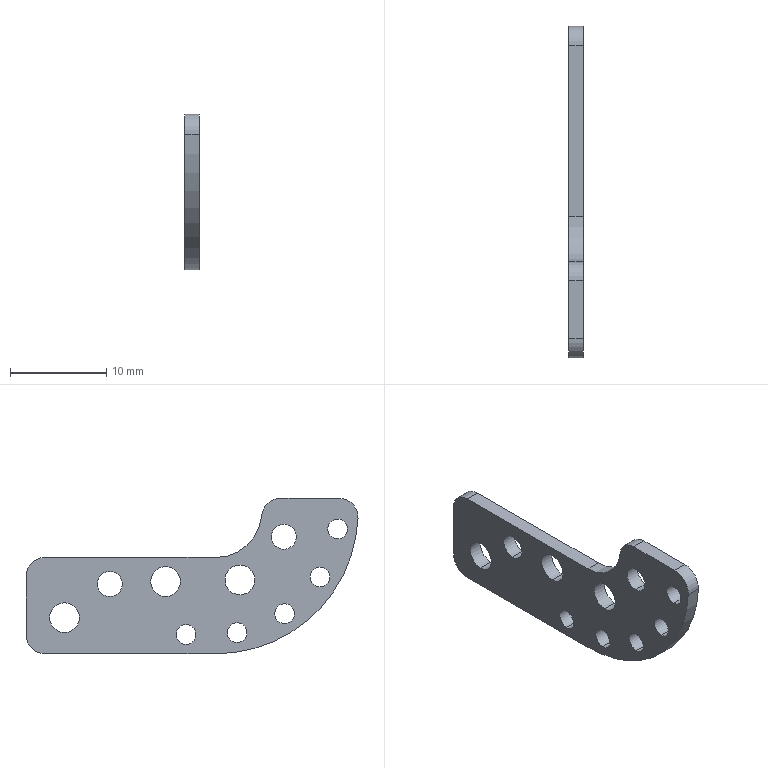Part | SolidWorks | features Extrusion 1, Fillet 1 | 1 solid | 32 faces | box 1.5 x 34.486 x 16.15 mm | volume 467.212 mm3 | cylinder 26 | plane 6 | commonest cylinder face diameters 2.05 x10 3.1 x6 2.6 x4 4 x4 9.5 x1 29.5 x1
STEP:
#1=CARTESIAN_POINT('',(1.5,5.25,15.2));
#2=VERTEX_POINT('',#1);
#3=CARTESIAN_POINT('',(1.5,5.25,18.3));
#4=VERTEX_POINT('',#3);
#5=CARTESIAN_POINT('',(1.5,5.25,16.75));
#6=DIRECTION('',(-1.,0.,0.));
#7=DIRECTION('',(0.,0.,-1.));
#8=AXIS2_PLACEMENT_3D('',#5,#6,#7);
#9=CIRCLE('',#8,1.55);
#10=EDGE_CURVE('',#2,#4,#9,.T.);
#11=ORIENTED_EDGE('',*,*,#10,.F.);
#12=CARTESIAN_POINT('',(0.,5.25,15.2));
#13=VERTEX_POINT('',#12);
#14=CARTESIAN_POINT('',(1.5,5.25,15.2));
#15=DIRECTION('',(-1.,0.,0.));
#16=VECTOR('',#15,1000.);
#17=LINE('',#14,#16);
#18=EDGE_CURVE('',#2,#13,#17,.T.);
#19=ORIENTED_EDGE('',*,*,#18,.T.);
#20=CARTESIAN_POINT('',(0.,5.25,18.3));
#21=VERTEX_POINT('',#20);
#22=CARTESIAN_POINT('',(0.,5.25,16.75));
#23=DIRECTION('',(-1.,0.,0.));
#24=DIRECTION('',(0.,0.,-1.));
#25=AXIS2_PLACEMENT_3D('',#22,#23,#24);
#26=CIRCLE('',#25,1.55);
#27=EDGE_CURVE('',#13,#21,#26,.T.);
#28=ORIENTED_EDGE('',*,*,#27,.T.);
#29=CARTESIAN_POINT('',(1.5,5.25,18.3));
#30=DIRECTION('',(-1.,0.,0.));
#31=VECTOR('',#30,1000.);
#32=LINE('',#29,#31);
#33=EDGE_CURVE('',#4,#21,#32,.T.);
#34=ORIENTED_EDGE('',*,*,#33,.F.);
#35=EDGE_LOOP('',(#11,#19,#28,#34));
#36=FACE_OUTER_BOUND('',#35,.T.);
#37=CARTESIAN_POINT('',(1.5,5.25,16.75));
#38=DIRECTION('',(-1.,0.,0.));
#39=DIRECTION('',(0.,0.,1.));
#40=AXIS2_PLACEMENT_3D('',#37,#38,#39);
#41=CYLINDRICAL_SURFACE('',#40,1.55);
#42=ADVANCED_FACE('',(#36),#41,.F.);
#43=CARTESIAN_POINT('',(1.5,15.75,14.55));
#44=VERTEX_POINT('',#43);
#45=CARTESIAN_POINT('',(1.5,15.75,11.45));
#46=VERTEX_POINT('',#45);
#47=CARTESIAN_POINT('',(1.5,15.75,13.));
#48=DIRECTION('',(1.,0.,0.));
#49=DIRECTION('',(0.,0.,-1.));
#50=AXIS2_PLACEMENT_3D('',#47,#48,#49);
#51=CIRCLE('',#50,1.55);
#52=EDGE_CURVE('',#44,#46,#51,.T.);
#53=ORIENTED_EDGE('',*,*,#52,.T.);
#54=CARTESIAN_POINT('',(0.,15.75,11.45));
#55=VERTEX_POINT('',#54);
#56=CARTESIAN_POINT('',(1.5,15.75,11.45));
#57=DIRECTION('',(-1.,0.,0.));
#58=VECTOR('',#57,1000.);
#59=LINE('',#56,#58);
#60=EDGE_CURVE('',#46,#55,#59,.T.);
#61=ORIENTED_EDGE('',*,*,#60,.T.);
#62=CARTESIAN_POINT('',(0.,15.75,14.55));
#63=VERTEX_POINT('',#62);
#64=CARTESIAN_POINT('',(0.,15.75,13.));
#65=DIRECTION('',(1.,0.,0.));
#66=DIRECTION('',(0.,0.,-1.));
#67=AXIS2_PLACEMENT_3D('',#64,#65,#66);
#68=CIRCLE('',#67,1.55);
#69=EDGE_CURVE('',#63,#55,#68,.T.);
#70=ORIENTED_EDGE('',*,*,#69,.F.);
#71=CARTESIAN_POINT('',(1.5,15.75,14.55));
#72=DIRECTION('',(-1.,0.,0.));
#73=VECTOR('',#72,1000.);
#74=LINE('',#71,#73);
#75=EDGE_CURVE('',#44,#63,#74,.T.);
#76=ORIENTED_EDGE('',*,*,#75,.F.);
#77=EDGE_LOOP('',(#53,#61,#70,#76));
#78=FACE_OUTER_BOUND('',#77,.T.);
#79=CARTESIAN_POINT('',(1.5,15.75,13.));
#80=DIRECTION('',(-1.,0.,0.));
#81=DIRECTION('',(0.,0.,1.));
#82=AXIS2_PLACEMENT_3D('',#79,#80,#81);
#83=CYLINDRICAL_SURFACE('',#82,1.55);
#84=ADVANCED_FACE('',(#78),#83,.F.);
#85=CARTESIAN_POINT('',(1.5,3.116,12.275));
#86=VERTEX_POINT('',#85);
#87=CARTESIAN_POINT('',(1.5,3.116,10.225));
#88=VERTEX_POINT('',#87);
#89=CARTESIAN_POINT('',(1.5,3.116,11.25));
#90=DIRECTION('',(1.,0.,0.));
#91=DIRECTION('',(0.,0.,-1.));
#92=AXIS2_PLACEMENT_3D('',#89,#90,#91);
#93=CIRCLE('',#92,1.025);
#94=EDGE_CURVE('',#86,#88,#93,.T.);
#95=ORIENTED_EDGE('',*,*,#94,.T.);
#96=CARTESIAN_POINT('',(0.,3.116,10.225));
#97=VERTEX_POINT('',#96);
#98=CARTESIAN_POINT('',(1.5,3.116,10.225));
#99=DIRECTION('',(-1.,0.,0.));
#100=VECTOR('',#99,1000.);
#101=LINE('',#98,#100);
#102=EDGE_CURVE('',#88,#97,#101,.T.);
#103=ORIENTED_EDGE('',*,*,#102,.T.);
#104=CARTESIAN_POINT('',(0.,3.116,12.275));
#105=VERTEX_POINT('',#104);
#106=CARTESIAN_POINT('',(0.,3.116,11.25));
#107=DIRECTION('',(1.,0.,0.));
#108=DIRECTION('',(0.,0.,-1.));
#109=AXIS2_PLACEMENT_3D('',#106,#107,#108);
#110=CIRCLE('',#109,1.025);
#111=EDGE_CURVE('',#105,#97,#110,.T.);
#112=ORIENTED_EDGE('',*,*,#111,.F.);
#113=CARTESIAN_POINT('',(1.5,3.116,12.275));
#114=DIRECTION('',(-1.,0.,0.));
#115=VECTOR('',#114,1000.);
#116=LINE('',#113,#115);
#117=EDGE_CURVE('',#86,#105,#116,.T.);
#118=ORIENTED_EDGE('',*,*,#117,.F.);
#119=EDGE_LOOP('',(#95,#103,#112,#118));
#120=FACE_OUTER_BOUND('',#119,.T.);
#121=CARTESIAN_POINT('',(1.5,3.116,11.25));
#122=DIRECTION('',(-1.,0.,0.));
#123=DIRECTION('',(0.,0.,1.));
#124=AXIS2_PLACEMENT_3D('',#121,#122,#123);
#125=CYLINDRICAL_SURFACE('',#124,1.025);
#126=ADVANCED_FACE('',(#120),#125,.F.);
#127=CARTESIAN_POINT('',(1.5,-12.621,23.219));
#128=VERTEX_POINT('',#127);
#129=CARTESIAN_POINT('',(1.5,-12.621,21.169));
#130=VERTEX_POINT('',#129);
#131=CARTESIAN_POINT('',(1.5,-12.621,22.194));
#132=DIRECTION('',(1.,0.,0.));
#133=DIRECTION('',(0.,0.,-1.));
#134=AXIS2_PLACEMENT_3D('',#131,#132,#133);
#135=CIRCLE('',#134,1.025);
#136=EDGE_CURVE('',#128,#130,#135,.T.);
#137=ORIENTED_EDGE('',*,*,#136,.T.);
#138=CARTESIAN_POINT('',(0.,-12.621,21.169));
#139=VERTEX_POINT('',#138);
#140=CARTESIAN_POINT('',(1.5,-12.621,21.169));
#141=DIRECTION('',(-1.,0.,0.));
#142=VECTOR('',#141,1000.);
#143=LINE('',#140,#142);
#144=EDGE_CURVE('',#130,#139,#143,.T.);
#145=ORIENTED_EDGE('',*,*,#144,.T.);
#146=CARTESIAN_POINT('',(0.,-12.621,23.219));
#147=VERTEX_POINT('',#146);
#148=CARTESIAN_POINT('',(0.,-12.621,22.194));
#149=DIRECTION('',(1.,0.,0.));
#150=DIRECTION('',(0.,0.,-1.));
#151=AXIS2_PLACEMENT_3D('',#148,#149,#150);
#152=CIRCLE('',#151,1.025);
#153=EDGE_CURVE('',#147,#139,#152,.T.);
#154=ORIENTED_EDGE('',*,*,#153,.F.);
#155=CARTESIAN_POINT('',(1.5,-12.621,23.219));
#156=DIRECTION('',(-1.,0.,0.));
#157=VECTOR('',#156,1000.);
#158=LINE('',#155,#157);
#159=EDGE_CURVE('',#128,#147,#158,.T.);
#160=ORIENTED_EDGE('',*,*,#159,.F.);
#161=EDGE_LOOP('',(#137,#145,#154,#160));
#162=FACE_OUTER_BOUND('',#161,.T.);
#163=CARTESIAN_POINT('',(1.5,-12.621,22.194));
#164=DIRECTION('',(-1.,0.,0.));
#165=DIRECTION('',(0.,0.,1.));
#166=AXIS2_PLACEMENT_3D('',#163,#164,#165);
#167=CYLINDRICAL_SURFACE('',#166,1.025);
#168=ADVANCED_FACE('',(#162),#167,.F.);
#169=CARTESIAN_POINT('',(1.5,-10.795,18.241));
#170=VERTEX_POINT('',#169);
#171=CARTESIAN_POINT('',(1.5,-10.795,16.191));
#172=VERTEX_POINT('',#171);
#173=CARTESIAN_POINT('',(1.5,-10.795,17.216));
#174=DIRECTION('',(1.,0.,0.));
#175=DIRECTION('',(0.,0.,-1.));
#176=AXIS2_PLACEMENT_3D('',#173,#174,#175);
#177=CIRCLE('',#176,1.025);
#178=EDGE_CURVE('',#170,#172,#177,.T.);
#179=ORIENTED_EDGE('',*,*,#178,.T.);
#180=CARTESIAN_POINT('',(0.,-10.795,16.191));
#181=VERTEX_POINT('',#180);
#182=CARTESIAN_POINT('',(1.5,-10.795,16.191));
#183=DIRECTION('',(-1.,0.,0.));
#184=VECTOR('',#183,1000.);
#185=LINE('',#182,#184);
#186=EDGE_CURVE('',#172,#181,#185,.T.);
#187=ORIENTED_EDGE('',*,*,#186,.T.);
#188=CARTESIAN_POINT('',(0.,-10.795,18.241));
#189=VERTEX_POINT('',#188);
#190=CARTESIAN_POINT('',(0.,-10.795,17.216));
#191=DIRECTION('',(1.,0.,0.));
#192=DIRECTION('',(0.,0.,-1.));
#193=AXIS2_PLACEMENT_3D('',#190,#191,#192);
#194=CIRCLE('',#193,1.025);
#195=EDGE_CURVE('',#189,#181,#194,.T.);
#196=ORIENTED_EDGE('',*,*,#195,.F.);
#197=CARTESIAN_POINT('',(1.5,-10.795,18.241));
#198=DIRECTION('',(-1.,0.,0.));
#199=VECTOR('',#198,1000.);
#200=LINE('',#197,#199);
#201=EDGE_CURVE('',#170,#189,#200,.T.);
#202=ORIENTED_EDGE('',*,*,#201,.F.);
#203=EDGE_LOOP('',(#179,#187,#196,#202));
#204=FACE_OUTER_BOUND('',#203,.T.);
#205=CARTESIAN_POINT('',(1.5,-10.795,17.216));
#206=DIRECTION('',(-1.,0.,0.));
#207=DIRECTION('',(0.,0.,1.));
#208=AXIS2_PLACEMENT_3D('',#205,#206,#207);
#209=CYLINDRICAL_SURFACE('',#208,1.025);
#210=ADVANCED_FACE('',(#204),#209,.F.);
#211=CARTESIAN_POINT('',(1.5,-7.103,14.437));
#212=VERTEX_POINT('',#211);
#213=CARTESIAN_POINT('',(1.5,-7.103,12.387));
#214=VERTEX_POINT('',#213);
#215=CARTESIAN_POINT('',(1.5,-7.103,13.412));
#216=DIRECTION('',(1.,0.,0.));
#217=DIRECTION('',(0.,0.,-1.));
#218=AXIS2_PLACEMENT_3D('',#215,#216,#217);
#219=CIRCLE('',#218,1.025);
#220=EDGE_CURVE('',#212,#214,#219,.T.);
#221=ORIENTED_EDGE('',*,*,#220,.T.);
#222=CARTESIAN_POINT('',(0.,-7.103,12.387));
#223=VERTEX_POINT('',#222);
#224=CARTESIAN_POINT('',(1.5,-7.103,12.387));
#225=DIRECTION('',(-1.,0.,0.));
#226=VECTOR('',#225,1000.);
#227=LINE('',#224,#226);
#228=EDGE_CURVE('',#214,#223,#227,.T.);
#229=ORIENTED_EDGE('',*,*,#228,.T.);
#230=CARTESIAN_POINT('',(0.,-7.103,14.437));
#231=VERTEX_POINT('',#230);
#232=CARTESIAN_POINT('',(0.,-7.103,13.412));
#233=DIRECTION('',(1.,0.,0.));
#234=DIRECTION('',(0.,0.,-1.));
#235=AXIS2_PLACEMENT_3D('',#232,#233,#234);
#236=CIRCLE('',#235,1.025);
#237=EDGE_CURVE('',#231,#223,#236,.T.);
#238=ORIENTED_EDGE('',*,*,#237,.F.);
#239=CARTESIAN_POINT('',(1.5,-7.103,14.437));
#240=DIRECTION('',(-1.,0.,0.));
#241=VECTOR('',#240,1000.);
#242=LINE('',#239,#241);
#243=EDGE_CURVE('',#212,#231,#242,.T.);
#244=ORIENTED_EDGE('',*,*,#243,.F.);
#245=EDGE_LOOP('',(#221,#229,#238,#244));
#246=FACE_OUTER_BOUND('',#245,.T.);
#247=CARTESIAN_POINT('',(1.5,-7.103,13.412));
#248=DIRECTION('',(-1.,0.,0.));
#249=DIRECTION('',(0.,0.,1.));
#250=AXIS2_PLACEMENT_3D('',#247,#248,#249);
#251=CYLINDRICAL_SURFACE('',#250,1.025);
#252=ADVANCED_FACE('',(#246),#251,.F.);
#253=CARTESIAN_POINT('',(1.5,-2.182,12.463));
#254=VERTEX_POINT('',#253);
#255=CARTESIAN_POINT('',(1.5,-2.182,10.413));
#256=VERTEX_POINT('',#255);
#257=CARTESIAN_POINT('',(1.5,-2.182,11.438));
#258=DIRECTION('',(1.,0.,0.));
#259=DIRECTION('',(0.,0.,-1.));
#260=AXIS2_PLACEMENT_3D('',#257,#258,#259);
#261=CIRCLE('',#260,1.025);
#262=EDGE_CURVE('',#254,#256,#261,.T.);
#263=ORIENTED_EDGE('',*,*,#262,.T.);
#264=CARTESIAN_POINT('',(0.,-2.182,10.413));
#265=VERTEX_POINT('',#264);
#266=CARTESIAN_POINT('',(1.5,-2.182,10.413));
#267=DIRECTION('',(-1.,0.,0.));
#268=VECTOR('',#267,1000.);
#269=LINE('',#266,#268);
#270=EDGE_CURVE('',#256,#265,#269,.T.);
#271=ORIENTED_EDGE('',*,*,#270,.T.);
#272=CARTESIAN_POINT('',(0.,-2.182,12.463));
#273=VERTEX_POINT('',#272);
#274=CARTESIAN_POINT('',(0.,-2.182,11.438));
#275=DIRECTION('',(1.,0.,0.));
#276=DIRECTION('',(0.,0.,-1.));
#277=AXIS2_PLACEMENT_3D('',#274,#275,#276);
#278=CIRCLE('',#277,1.025);
#279=EDGE_CURVE('',#273,#265,#278,.T.);
#280=ORIENTED_EDGE('',*,*,#279,.F.);
#281=CARTESIAN_POINT('',(1.5,-2.182,12.463));
#282=DIRECTION('',(-1.,0.,0.));
#283=VECTOR('',#282,1000.);
#284=LINE('',#281,#283);
#285=EDGE_CURVE('',#254,#273,#284,.T.);
#286=ORIENTED_EDGE('',*,*,#285,.F.);
#287=EDGE_LOOP('',(#263,#271,#280,#286));
#288=FACE_OUTER_BOUND('',#287,.T.);
#289=CARTESIAN_POINT('',(1.5,-2.182,11.438));
#290=DIRECTION('',(-1.,0.,0.));
#291=DIRECTION('',(0.,0.,1.));
#292=AXIS2_PLACEMENT_3D('',#289,#290,#291);
#293=CYLINDRICAL_SURFACE('',#292,1.025);
#294=ADVANCED_FACE('',(#288),#293,.F.);
#295=CARTESIAN_POINT('',(1.5,11.05,17.8));
#296=VERTEX_POINT('',#295);
#297=CARTESIAN_POINT('',(1.5,11.05,15.2));
#298=VERTEX_POINT('',#297);
#299=CARTESIAN_POINT('',(1.5,11.05,16.5));
#300=DIRECTION('',(1.,0.,0.));
#301=DIRECTION('',(0.,0.,-1.));
#302=AXIS2_PLACEMENT_3D('',#299,#300,#301);
#303=CIRCLE('',#302,1.3);
#304=EDGE_CURVE('',#296,#298,#303,.T.);
#305=ORIENTED_EDGE('',*,*,#304,.T.);
#306=CARTESIAN_POINT('',(0.,11.05,15.2));
#307=VERTEX_POINT('',#306);
#308=CARTESIAN_POINT('',(1.5,11.05,15.2));
#309=DIRECTION('',(-1.,0.,0.));
#310=VECTOR('',#309,1000.);
#311=LINE('',#308,#310);
#312=EDGE_CURVE('',#298,#307,#311,.T.);
#313=ORIENTED_EDGE('',*,*,#312,.T.);
#314=CARTESIAN_POINT('',(0.,11.05,17.8));
#315=VERTEX_POINT('',#314);
#316=CARTESIAN_POINT('',(0.,11.05,16.5));
#317=DIRECTION('',(1.,0.,0.));
#318=DIRECTION('',(0.,0.,-1.));
#319=AXIS2_PLACEMENT_3D('',#316,#317,#318);
#320=CIRCLE('',#319,1.3);
#321=EDGE_CURVE('',#315,#307,#320,.T.);
#322=ORIENTED_EDGE('',*,*,#321,.F.);
#323=CARTESIAN_POINT('',(1.5,11.05,17.8));
#324=DIRECTION('',(-1.,0.,0.));
#325=VECTOR('',#324,1000.);
#326=LINE('',#323,#325);
#327=EDGE_CURVE('',#296,#315,#326,.T.);
#328=ORIENTED_EDGE('',*,*,#327,.F.);
#329=EDGE_LOOP('',(#305,#313,#322,#328));
#330=FACE_OUTER_BOUND('',#329,.T.);
#331=CARTESIAN_POINT('',(1.5,11.05,16.5));
#332=DIRECTION('',(-1.,0.,0.));
#333=DIRECTION('',(0.,0.,1.));
#334=AXIS2_PLACEMENT_3D('',#331,#332,#333);
#335=CYLINDRICAL_SURFACE('',#334,1.3);
#336=ADVANCED_FACE('',(#330),#335,.F.);
#337=CARTESIAN_POINT('',(1.5,-7.035,22.7));
#338=VERTEX_POINT('',#337);
#339=CARTESIAN_POINT('',(1.5,-7.035,20.1));
#340=VERTEX_POINT('',#339);
#341=CARTESIAN_POINT('',(1.5,-7.035,21.4));
#342=DIRECTION('',(1.,0.,0.));
#343=DIRECTION('',(0.,0.,-1.));
#344=AXIS2_PLACEMENT_3D('',#341,#342,#343);
#345=CIRCLE('',#344,1.3);
#346=EDGE_CURVE('',#338,#340,#345,.T.);
#347=ORIENTED_EDGE('',*,*,#346,.T.);
#348=CARTESIAN_POINT('',(0.,-7.035,20.1));
#349=VERTEX_POINT('',#348);
#350=CARTESIAN_POINT('',(1.5,-7.035,20.1));
#351=DIRECTION('',(-1.,0.,0.));
#352=VECTOR('',#351,1000.);
#353=LINE('',#350,#352);
#354=EDGE_CURVE('',#340,#349,#353,.T.);
#355=ORIENTED_EDGE('',*,*,#354,.T.);
#356=CARTESIAN_POINT('',(0.,-7.035,22.7));
#357=VERTEX_POINT('',#356);
#358=CARTESIAN_POINT('',(0.,-7.035,21.4));
#359=DIRECTION('',(1.,0.,0.));
#360=DIRECTION('',(0.,0.,-1.));
#361=AXIS2_PLACEMENT_3D('',#358,#359,#360);
#362=CIRCLE('',#361,1.3);
#363=EDGE_CURVE('',#357,#349,#362,.T.);
#364=ORIENTED_EDGE('',*,*,#363,.F.);
#365=CARTESIAN_POINT('',(1.5,-7.035,22.7));
#366=DIRECTION('',(-1.,0.,0.));
#367=VECTOR('',#366,1000.);
#368=LINE('',#365,#367);
#369=EDGE_CURVE('',#338,#357,#368,.T.);
#370=ORIENTED_EDGE('',*,*,#369,.F.);
#371=EDGE_LOOP('',(#347,#355,#364,#370));
#372=FACE_OUTER_BOUND('',#371,.T.);
#373=CARTESIAN_POINT('',(1.5,-7.035,21.4));
#374=DIRECTION('',(-1.,0.,0.));
#375=DIRECTION('',(0.,0.,1.));
#376=AXIS2_PLACEMENT_3D('',#373,#374,#375);
#377=CYLINDRICAL_SURFACE('',#376,1.3);
#378=ADVANCED_FACE('',(#372),#377,.F.);
#379=CARTESIAN_POINT('',(1.5,-2.467,18.467));
#380=VERTEX_POINT('',#379);
#381=CARTESIAN_POINT('',(1.5,-2.467,15.367));
#382=VERTEX_POINT('',#381);
#383=CARTESIAN_POINT('',(1.5,-2.467,16.917));
#384=DIRECTION('',(1.,0.,0.));
#385=DIRECTION('',(0.,0.,-1.));
#386=AXIS2_PLACEMENT_3D('',#383,#384,#385);
#387=CIRCLE('',#386,1.55);
#388=EDGE_CURVE('',#380,#382,#387,.T.);
#389=ORIENTED_EDGE('',*,*,#388,.T.);
#390=CARTESIAN_POINT('',(0.,-2.467,15.367));
#391=VERTEX_POINT('',#390);
#392=CARTESIAN_POINT('',(1.5,-2.467,15.367));
#393=DIRECTION('',(-1.,0.,0.));
#394=VECTOR('',#393,1000.);
#395=LINE('',#392,#394);
#396=EDGE_CURVE('',#382,#391,#395,.T.);
#397=ORIENTED_EDGE('',*,*,#396,.T.);
#398=CARTESIAN_POINT('',(0.,-2.467,18.467));
#399=VERTEX_POINT('',#398);
#400=CARTESIAN_POINT('',(0.,-2.467,16.917));
#401=DIRECTION('',(1.,0.,0.));
#402=DIRECTION('',(0.,0.,-1.));
#403=AXIS2_PLACEMENT_3D('',#400,#401,#402);
#404=CIRCLE('',#403,1.55);
#405=EDGE_CURVE('',#399,#391,#404,.T.);
#406=ORIENTED_EDGE('',*,*,#405,.F.);
#407=CARTESIAN_POINT('',(1.5,-2.467,18.467));
#408=DIRECTION('',(-1.,0.,0.));
#409=VECTOR('',#408,1000.);
#410=LINE('',#407,#409);
#411=EDGE_CURVE('',#380,#399,#410,.T.);
#412=ORIENTED_EDGE('',*,*,#411,.F.);
#413=EDGE_LOOP('',(#389,#397,#406,#412));
#414=FACE_OUTER_BOUND('',#413,.T.);
#415=CARTESIAN_POINT('',(1.5,-2.467,16.917));
#416=DIRECTION('',(-1.,0.,0.));
#417=DIRECTION('',(0.,0.,1.));
#418=AXIS2_PLACEMENT_3D('',#415,#416,#417);
#419=CYLINDRICAL_SURFACE('',#418,1.55);
#420=ADVANCED_FACE('',(#414),#419,.F.);
#421=CARTESIAN_POINT('',(0.,0.,9.25));
#422=VERTEX_POINT('',#421);
#423=CARTESIAN_POINT('',(0.,17.75,9.25));
#424=VERTEX_POINT('',#423);
#425=CARTESIAN_POINT('',(0.,0.,9.25));
#426=DIRECTION('',(0.,1.,0.));
#427=VECTOR('',#426,1000.);
#428=LINE('',#425,#427);
#429=EDGE_CURVE('',#422,#424,#428,.T.);
#430=ORIENTED_EDGE('',*,*,#429,.T.);
#431=CARTESIAN_POINT('',(1.5,17.75,9.25));
#432=VERTEX_POINT('',#431);
#433=CARTESIAN_POINT('',(1.5,17.75,9.25));
#434=DIRECTION('',(1.,0.,0.));
#435=VECTOR('',#434,1000.);
#436=LINE('',#433,#435);
#437=EDGE_CURVE('',#424,#432,#436,.T.);
#438=ORIENTED_EDGE('',*,*,#437,.T.);
#439=CARTESIAN_POINT('',(1.5,0.,9.25));
#440=VERTEX_POINT('',#439);
#441=CARTESIAN_POINT('',(1.5,0.,9.25));
#442=DIRECTION('',(0.,1.,0.));
#443=VECTOR('',#442,1000.);
#444=LINE('',#441,#443);
#445=EDGE_CURVE('',#440,#432,#444,.T.);
#446=ORIENTED_EDGE('',*,*,#445,.F.);
#447=CARTESIAN_POINT('',(1.5,0.,9.25));
#448=DIRECTION('',(-1.,0.,0.));
#449=VECTOR('',#448,1000.);
#450=LINE('',#447,#449);
#451=EDGE_CURVE('',#440,#422,#450,.T.);
#452=ORIENTED_EDGE('',*,*,#451,.T.);
#453=EDGE_LOOP('',(#430,#438,#446,#452));
#454=FACE_OUTER_BOUND('',#453,.T.);
#455=CARTESIAN_POINT('',(1.5,0.,9.25));
#456=DIRECTION('',(0.,0.,1.));
#457=DIRECTION('',(1.,0.,0.));
#458=AXIS2_PLACEMENT_3D('',#455,#456,#457);
#459=PLANE('',#458);
#460=ADVANCED_FACE('',(#454),#459,.F.);
#461=CARTESIAN_POINT('',(0.,19.75,17.25));
#462=VERTEX_POINT('',#461);
#463=CARTESIAN_POINT('',(0.,19.75,11.25));
#464=VERTEX_POINT('',#463);
#465=CARTESIAN_POINT('',(0.,19.75,0.));
#466=DIRECTION('',(0.,0.,-1.));
#467=VECTOR('',#466,1000.);
#468=LINE('',#465,#467);
#469=EDGE_CURVE('',#462,#464,#468,.T.);
#470=ORIENTED_EDGE('',*,*,#469,.F.);
#471=CARTESIAN_POINT('',(1.5,19.75,17.25));
#472=VERTEX_POINT('',#471);
#473=CARTESIAN_POINT('',(1.5,19.75,17.25));
#474=DIRECTION('',(1.,0.,0.));
#475=VECTOR('',#474,1000.);
#476=LINE('',#473,#475);
#477=EDGE_CURVE('',#462,#472,#476,.T.);
#478=ORIENTED_EDGE('',*,*,#477,.T.);
#479=CARTESIAN_POINT('',(1.5,19.75,11.25));
#480=VERTEX_POINT('',#479);
#481=CARTESIAN_POINT('',(1.5,19.75,0.));
#482=DIRECTION('',(0.,0.,-1.));
#483=VECTOR('',#482,1000.);
#484=LINE('',#481,#483);
#485=EDGE_CURVE('',#472,#480,#484,.T.);
#486=ORIENTED_EDGE('',*,*,#485,.T.);
#487=CARTESIAN_POINT('',(0.,19.75,11.25));
#488=DIRECTION('',(-1.,0.,0.));
#489=VECTOR('',#488,1000.);
#490=LINE('',#487,#489);
#491=EDGE_CURVE('',#480,#464,#490,.T.);
#492=ORIENTED_EDGE('',*,*,#491,.T.);
#493=EDGE_LOOP('',(#470,#478,#486,#492));
#494=FACE_OUTER_BOUND('',#493,.T.);
#495=CARTESIAN_POINT('',(1.5,19.75,0.));
#496=DIRECTION('',(0.,1.,0.));
#497=DIRECTION('',(0.,0.,1.));
#498=AXIS2_PLACEMENT_3D('',#495,#496,#497);
#499=PLANE('',#498);
#500=ADVANCED_FACE('',(#494),#499,.T.);
#501=CARTESIAN_POINT('',(1.5,0.,19.25));
#502=VERTEX_POINT('',#501);
#503=CARTESIAN_POINT('',(1.5,17.75,19.25));
#504=VERTEX_POINT('',#503);
#505=CARTESIAN_POINT('',(1.5,0.,19.25));
#506=DIRECTION('',(0.,1.,0.));
#507=VECTOR('',#506,1000.);
#508=LINE('',#505,#507);
#509=EDGE_CURVE('',#502,#504,#508,.T.);
#510=ORIENTED_EDGE('',*,*,#509,.T.);
#511=CARTESIAN_POINT('',(0.,17.75,19.25));
#512=VERTEX_POINT('',#511);
#513=CARTESIAN_POINT('',(1.5,17.75,19.25));
#514=DIRECTION('',(-1.,0.,0.));
#515=VECTOR('',#514,1000.);
#516=LINE('',#513,#515);
#517=EDGE_CURVE('',#504,#512,#516,.T.);
#518=ORIENTED_EDGE('',*,*,#517,.T.);
#519=CARTESIAN_POINT('',(0.,0.,19.25));
#520=VERTEX_POINT('',#519);
#521=CARTESIAN_POINT('',(0.,0.,19.25));
#522=DIRECTION('',(0.,1.,0.));
#523=VECTOR('',#522,1000.);
#524=LINE('',#521,#523);
#525=EDGE_CURVE('',#520,#512,#524,.T.);
#526=ORIENTED_EDGE('',*,*,#525,.F.);
#527=CARTESIAN_POINT('',(1.5,0.,19.25));
#528=DIRECTION('',(-1.,0.,0.));
#529=VECTOR('',#528,1000.);
#530=LINE('',#527,#529);
#531=EDGE_CURVE('',#502,#520,#530,.T.);
#532=ORIENTED_EDGE('',*,*,#531,.F.);
#533=EDGE_LOOP('',(#510,#518,#526,#532));
#534=FACE_OUTER_BOUND('',#533,.T.);
#535=CARTESIAN_POINT('',(1.5,0.,19.25));
#536=DIRECTION('',(0.,0.,1.));
#537=DIRECTION('',(0.,-1.,0.));
#538=AXIS2_PLACEMENT_3D('',#535,#536,#537);
#539=PLANE('',#538);
#540=ADVANCED_FACE('',(#534),#539,.T.);
#541=CARTESIAN_POINT('',(0.,-4.731,23.578));
#542=VERTEX_POINT('',#541);
#543=CARTESIAN_POINT('',(0.,0.,24.));
#544=DIRECTION('',(1.,0.,0.));
#545=DIRECTION('',(0.,0.,-1.));
#546=AXIS2_PLACEMENT_3D('',#543,#544,#545);
#547=CIRCLE('',#546,4.75);
#548=EDGE_CURVE('',#542,#520,#547,.T.);
#549=ORIENTED_EDGE('',*,*,#548,.F.);
#550=CARTESIAN_POINT('',(1.5,-4.731,23.578));
#551=VERTEX_POINT('',#550);
#552=CARTESIAN_POINT('',(1.5,-4.731,23.578));
#553=DIRECTION('',(1.,0.,0.));
#554=VECTOR('',#553,1000.);
#555=LINE('',#552,#554);
#556=EDGE_CURVE('',#542,#551,#555,.T.);
#557=ORIENTED_EDGE('',*,*,#556,.T.);
#558=CARTESIAN_POINT('',(1.5,0.,24.));
#559=DIRECTION('',(1.,0.,0.));
#560=DIRECTION('',(0.,0.,-1.));
#561=AXIS2_PLACEMENT_3D('',#558,#559,#560);
#562=CIRCLE('',#561,4.75);
#563=EDGE_CURVE('',#551,#502,#562,.T.);
#564=ORIENTED_EDGE('',*,*,#563,.T.);
#565=ORIENTED_EDGE('',*,*,#531,.T.);
#566=EDGE_LOOP('',(#549,#557,#564,#565));
#567=FACE_OUTER_BOUND('',#566,.T.);
#568=CARTESIAN_POINT('',(1.5,0.,24.));
#569=DIRECTION('',(-1.,0.,0.));
#570=DIRECTION('',(0.,0.,1.));
#571=AXIS2_PLACEMENT_3D('',#568,#569,#570);
#572=CYLINDRICAL_SURFACE('',#571,4.75);
#573=ADVANCED_FACE('',(#567),#572,.F.);
#574=CARTESIAN_POINT('',(1.5,-6.723,25.4));
#575=VERTEX_POINT('',#574);
#576=CARTESIAN_POINT('',(1.5,-12.736,25.4));
#577=VERTEX_POINT('',#576);
#578=CARTESIAN_POINT('',(1.5,0.,25.4));
#579=DIRECTION('',(0.,-1.,0.));
#580=VECTOR('',#579,1000.);
#581=LINE('',#578,#580);
#582=EDGE_CURVE('',#575,#577,#581,.T.);
#583=ORIENTED_EDGE('',*,*,#582,.F.);
#584=CARTESIAN_POINT('',(0.,-6.723,25.4));
#585=VERTEX_POINT('',#584);
#586=CARTESIAN_POINT('',(0.,-6.723,25.4));
#587=DIRECTION('',(-1.,0.,0.));
#588=VECTOR('',#587,1000.);
#589=LINE('',#586,#588);
#590=EDGE_CURVE('',#575,#585,#589,.T.);
#591=ORIENTED_EDGE('',*,*,#590,.T.);
#592=CARTESIAN_POINT('',(0.,-12.736,25.4));
#593=VERTEX_POINT('',#592);
#594=CARTESIAN_POINT('',(0.,0.,25.4));
#595=DIRECTION('',(0.,-1.,0.));
#596=VECTOR('',#595,1000.);
#597=LINE('',#594,#596);
#598=EDGE_CURVE('',#585,#593,#597,.T.);
#599=ORIENTED_EDGE('',*,*,#598,.T.);
#600=CARTESIAN_POINT('',(1.5,-12.736,25.4));
#601=DIRECTION('',(1.,0.,0.));
#602=VECTOR('',#601,1000.);
#603=LINE('',#600,#602);
#604=EDGE_CURVE('',#593,#577,#603,.T.);
#605=ORIENTED_EDGE('',*,*,#604,.T.);
#606=EDGE_LOOP('',(#583,#591,#599,#605));
#607=FACE_OUTER_BOUND('',#606,.T.);
#608=CARTESIAN_POINT('',(1.5,0.,25.4));
#609=DIRECTION('',(0.,0.,-1.));
#610=DIRECTION('',(0.,1.,0.));
#611=AXIS2_PLACEMENT_3D('',#608,#609,#610);
#612=PLANE('',#611);
#613=ADVANCED_FACE('',(#607),#612,.F.);
#614=ORIENTED_EDGE('',*,*,#396,.F.);
#615=CARTESIAN_POINT('',(1.5,-2.467,16.917));
#616=DIRECTION('',(1.,0.,0.));
#617=DIRECTION('',(0.,0.,-1.));
#618=AXIS2_PLACEMENT_3D('',#615,#616,#617);
#619=CIRCLE('',#618,1.55);
#620=EDGE_CURVE('',#382,#380,#619,.T.);
#621=ORIENTED_EDGE('',*,*,#620,.T.);
#622=ORIENTED_EDGE('',*,*,#411,.T.);
#623=CARTESIAN_POINT('',(0.,-2.467,16.917));
#624=DIRECTION('',(1.,0.,0.));
#625=DIRECTION('',(0.,0.,-1.));
#626=AXIS2_PLACEMENT_3D('',#623,#624,#625);
#627=CIRCLE('',#626,1.55);
#628=EDGE_CURVE('',#391,#399,#627,.T.);
#629=ORIENTED_EDGE('',*,*,#628,.F.);
#630=EDGE_LOOP('',(#614,#621,#622,#629));
#631=FACE_OUTER_BOUND('',#630,.T.);
#632=CARTESIAN_POINT('',(1.5,-2.467,16.917));
#633=DIRECTION('',(-1.,0.,0.));
#634=DIRECTION('',(0.,0.,1.));
#635=AXIS2_PLACEMENT_3D('',#632,#633,#634);
#636=CYLINDRICAL_SURFACE('',#635,1.55);
#637=ADVANCED_FACE('',(#631),#636,.F.);
#638=ORIENTED_EDGE('',*,*,#354,.F.);
#639=CARTESIAN_POINT('',(1.5,-7.035,21.4));
#640=DIRECTION('',(1.,0.,0.));
#641=DIRECTION('',(0.,0.,-1.));
#642=AXIS2_PLACEMENT_3D('',#639,#640,#641);
#643=CIRCLE('',#642,1.3);
#644=EDGE_CURVE('',#340,#338,#643,.T.);
#645=ORIENTED_EDGE('',*,*,#644,.T.);
#646=ORIENTED_EDGE('',*,*,#369,.T.);
#647=CARTESIAN_POINT('',(0.,-7.035,21.4));
#648=DIRECTION('',(1.,0.,0.));
#649=DIRECTION('',(0.,0.,-1.));
#650=AXIS2_PLACEMENT_3D('',#647,#648,#649);
#651=CIRCLE('',#650,1.3);
#652=EDGE_CURVE('',#349,#357,#651,.T.);
#653=ORIENTED_EDGE('',*,*,#652,.F.);
#654=EDGE_LOOP('',(#638,#645,#646,#653));
#655=FACE_OUTER_BOUND('',#654,.T.);
#656=CARTESIAN_POINT('',(1.5,-7.035,21.4));
#657=DIRECTION('',(-1.,0.,0.));
#658=DIRECTION('',(0.,0.,1.));
#659=AXIS2_PLACEMENT_3D('',#656,#657,#658);
#660=CYLINDRICAL_SURFACE('',#659,1.3);
#661=ADVANCED_FACE('',(#655),#660,.F.);
#662=ORIENTED_EDGE('',*,*,#312,.F.);
#663=CARTESIAN_POINT('',(1.5,11.05,16.5));
#664=DIRECTION('',(1.,0.,0.));
#665=DIRECTION('',(0.,0.,-1.));
#666=AXIS2_PLACEMENT_3D('',#663,#664,#665);
#667=CIRCLE('',#666,1.3);
#668=EDGE_CURVE('',#298,#296,#667,.T.);
#669=ORIENTED_EDGE('',*,*,#668,.T.);
#670=ORIENTED_EDGE('',*,*,#327,.T.);
#671=CARTESIAN_POINT('',(0.,11.05,16.5));
#672=DIRECTION('',(1.,0.,0.));
#673=DIRECTION('',(0.,0.,-1.));
#674=AXIS2_PLACEMENT_3D('',#671,#672,#673);
#675=CIRCLE('',#674,1.3);
#676=EDGE_CURVE('',#307,#315,#675,.T.);
#677=ORIENTED_EDGE('',*,*,#676,.F.);
#678=EDGE_LOOP('',(#662,#669,#670,#677));
#679=FACE_OUTER_BOUND('',#678,.T.);
#680=CARTESIAN_POINT('',(1.5,11.05,16.5));
#681=DIRECTION('',(-1.,0.,0.));
#682=DIRECTION('',(0.,0.,1.));
#683=AXIS2_PLACEMENT_3D('',#680,#681,#682);
#684=CYLINDRICAL_SURFACE('',#683,1.3);
#685=ADVANCED_FACE('',(#679),#684,.F.);
#686=ORIENTED_EDGE('',*,*,#270,.F.);
#687=CARTESIAN_POINT('',(1.5,-2.182,11.438));
#688=DIRECTION('',(1.,0.,0.));
#689=DIRECTION('',(0.,0.,-1.));
#690=AXIS2_PLACEMENT_3D('',#687,#688,#689);
#691=CIRCLE('',#690,1.025);
#692=EDGE_CURVE('',#256,#254,#691,.T.);
#693=ORIENTED_EDGE('',*,*,#692,.T.);
#694=ORIENTED_EDGE('',*,*,#285,.T.);
#695=CARTESIAN_POINT('',(0.,-2.182,11.438));
#696=DIRECTION('',(1.,0.,0.));
#697=DIRECTION('',(0.,0.,-1.));
#698=AXIS2_PLACEMENT_3D('',#695,#696,#697);
#699=CIRCLE('',#698,1.025);
#700=EDGE_CURVE('',#265,#273,#699,.T.);
#701=ORIENTED_EDGE('',*,*,#700,.F.);
#702=EDGE_LOOP('',(#686,#693,#694,#701));
#703=FACE_OUTER_BOUND('',#702,.T.);
#704=CARTESIAN_POINT('',(1.5,-2.182,11.438));
#705=DIRECTION('',(-1.,0.,0.));
#706=DIRECTION('',(0.,0.,1.));
#707=AXIS2_PLACEMENT_3D('',#704,#705,#706);
#708=CYLINDRICAL_SURFACE('',#707,1.025);
#709=ADVANCED_FACE('',(#703),#708,.F.);
#710=ORIENTED_EDGE('',*,*,#228,.F.);
#711=CARTESIAN_POINT('',(1.5,-7.103,13.412));
#712=DIRECTION('',(1.,0.,0.));
#713=DIRECTION('',(0.,0.,-1.));
#714=AXIS2_PLACEMENT_3D('',#711,#712,#713);
#715=CIRCLE('',#714,1.025);
#716=EDGE_CURVE('',#214,#212,#715,.T.);
#717=ORIENTED_EDGE('',*,*,#716,.T.);
#718=ORIENTED_EDGE('',*,*,#243,.T.);
#719=CARTESIAN_POINT('',(0.,-7.103,13.412));
#720=DIRECTION('',(1.,0.,0.));
#721=DIRECTION('',(0.,0.,-1.));
#722=AXIS2_PLACEMENT_3D('',#719,#720,#721);
#723=CIRCLE('',#722,1.025);
#724=EDGE_CURVE('',#223,#231,#723,.T.);
#725=ORIENTED_EDGE('',*,*,#724,.F.);
#726=EDGE_LOOP('',(#710,#717,#718,#725));
#727=FACE_OUTER_BOUND('',#726,.T.);
#728=CARTESIAN_POINT('',(1.5,-7.103,13.412));
#729=DIRECTION('',(-1.,0.,0.));
#730=DIRECTION('',(0.,0.,1.));
#731=AXIS2_PLACEMENT_3D('',#728,#729,#730);
#732=CYLINDRICAL_SURFACE('',#731,1.025);
#733=ADVANCED_FACE('',(#727),#732,.F.);
#734=ORIENTED_EDGE('',*,*,#186,.F.);
#735=CARTESIAN_POINT('',(1.5,-10.795,17.216));
#736=DIRECTION('',(1.,0.,0.));
#737=DIRECTION('',(0.,0.,-1.));
#738=AXIS2_PLACEMENT_3D('',#735,#736,#737);
#739=CIRCLE('',#738,1.025);
#740=EDGE_CURVE('',#172,#170,#739,.T.);
#741=ORIENTED_EDGE('',*,*,#740,.T.);
#742=ORIENTED_EDGE('',*,*,#201,.T.);
#743=CARTESIAN_POINT('',(0.,-10.795,17.216));
#744=DIRECTION('',(1.,0.,0.));
#745=DIRECTION('',(0.,0.,-1.));
#746=AXIS2_PLACEMENT_3D('',#743,#744,#745);
#747=CIRCLE('',#746,1.025);
#748=EDGE_CURVE('',#181,#189,#747,.T.);
#749=ORIENTED_EDGE('',*,*,#748,.F.);
#750=EDGE_LOOP('',(#734,#741,#742,#749));
#751=FACE_OUTER_BOUND('',#750,.T.);
#752=CARTESIAN_POINT('',(1.5,-10.795,17.216));
#753=DIRECTION('',(-1.,0.,0.));
#754=DIRECTION('',(0.,0.,1.));
#755=AXIS2_PLACEMENT_3D('',#752,#753,#754);
#756=CYLINDRICAL_SURFACE('',#755,1.025);
#757=ADVANCED_FACE('',(#751),#756,.F.);
#758=ORIENTED_EDGE('',*,*,#144,.F.);
#759=CARTESIAN_POINT('',(1.5,-12.621,22.194));
#760=DIRECTION('',(1.,0.,0.));
#761=DIRECTION('',(0.,0.,-1.));
#762=AXIS2_PLACEMENT_3D('',#759,#760,#761);
#763=CIRCLE('',#762,1.025);
#764=EDGE_CURVE('',#130,#128,#763,.T.);
#765=ORIENTED_EDGE('',*,*,#764,.T.);
#766=ORIENTED_EDGE('',*,*,#159,.T.);
#767=CARTESIAN_POINT('',(0.,-12.621,22.194));
#768=DIRECTION('',(1.,0.,0.));
#769=DIRECTION('',(0.,0.,-1.));
#770=AXIS2_PLACEMENT_3D('',#767,#768,#769);
#771=CIRCLE('',#770,1.025);
#772=EDGE_CURVE('',#139,#147,#771,.T.);
#773=ORIENTED_EDGE('',*,*,#772,.F.);
#774=EDGE_LOOP('',(#758,#765,#766,#773));
#775=FACE_OUTER_BOUND('',#774,.T.);
#776=CARTESIAN_POINT('',(1.5,-12.621,22.194));
#777=DIRECTION('',(-1.,0.,0.));
#778=DIRECTION('',(0.,0.,1.));
#779=AXIS2_PLACEMENT_3D('',#776,#777,#778);
#780=CYLINDRICAL_SURFACE('',#779,1.025);
#781=ADVANCED_FACE('',(#775),#780,.F.);
#782=ORIENTED_EDGE('',*,*,#102,.F.);
#783=CARTESIAN_POINT('',(1.5,3.116,11.25));
#784=DIRECTION('',(1.,0.,0.));
#785=DIRECTION('',(0.,0.,-1.));
#786=AXIS2_PLACEMENT_3D('',#783,#784,#785);
#787=CIRCLE('',#786,1.025);
#788=EDGE_CURVE('',#88,#86,#787,.T.);
#789=ORIENTED_EDGE('',*,*,#788,.T.);
#790=ORIENTED_EDGE('',*,*,#117,.T.);
#791=CARTESIAN_POINT('',(0.,3.116,11.25));
#792=DIRECTION('',(1.,0.,0.));
#793=DIRECTION('',(0.,0.,-1.));
#794=AXIS2_PLACEMENT_3D('',#791,#792,#793);
#795=CIRCLE('',#794,1.025);
#796=EDGE_CURVE('',#97,#105,#795,.T.);
#797=ORIENTED_EDGE('',*,*,#796,.F.);
#798=EDGE_LOOP('',(#782,#789,#790,#797));
#799=FACE_OUTER_BOUND('',#798,.T.);
#800=CARTESIAN_POINT('',(1.5,3.116,11.25));
#801=DIRECTION('',(-1.,0.,0.));
#802=DIRECTION('',(0.,0.,1.));
#803=AXIS2_PLACEMENT_3D('',#800,#801,#802);
#804=CYLINDRICAL_SURFACE('',#803,1.025);
#805=ADVANCED_FACE('',(#799),#804,.F.);
#806=ORIENTED_EDGE('',*,*,#60,.F.);
#807=CARTESIAN_POINT('',(1.5,15.75,13.));
#808=DIRECTION('',(1.,0.,0.));
#809=DIRECTION('',(0.,0.,-1.));
#810=AXIS2_PLACEMENT_3D('',#807,#808,#809);
#811=CIRCLE('',#810,1.55);
#812=EDGE_CURVE('',#46,#44,#811,.T.);
#813=ORIENTED_EDGE('',*,*,#812,.T.);
#814=ORIENTED_EDGE('',*,*,#75,.T.);
#815=CARTESIAN_POINT('',(0.,15.75,13.));
#816=DIRECTION('',(1.,0.,0.));
#817=DIRECTION('',(0.,0.,-1.));
#818=AXIS2_PLACEMENT_3D('',#815,#816,#817);
#819=CIRCLE('',#818,1.55);
#820=EDGE_CURVE('',#55,#63,#819,.T.);
#821=ORIENTED_EDGE('',*,*,#820,.F.);
#822=EDGE_LOOP('',(#806,#813,#814,#821));
#823=FACE_OUTER_BOUND('',#822,.T.);
#824=CARTESIAN_POINT('',(1.5,15.75,13.));
#825=DIRECTION('',(-1.,0.,0.));
#826=DIRECTION('',(0.,0.,1.));
#827=AXIS2_PLACEMENT_3D('',#824,#825,#826);
#828=CYLINDRICAL_SURFACE('',#827,1.55);
#829=ADVANCED_FACE('',(#823),#828,.F.);
#830=CARTESIAN_POINT('',(1.5,-14.734,23.306));
#831=VERTEX_POINT('',#830);
#832=CARTESIAN_POINT('',(1.5,0.,24.));
#833=DIRECTION('',(1.,0.,0.));
#834=DIRECTION('',(0.,0.,-1.));
#835=AXIS2_PLACEMENT_3D('',#832,#833,#834);
#836=CIRCLE('',#835,14.75);
#837=EDGE_CURVE('',#831,#440,#836,.T.);
#838=ORIENTED_EDGE('',*,*,#837,.F.);
#839=CARTESIAN_POINT('',(0.,-14.734,23.306));
#840=VERTEX_POINT('',#839);
#841=CARTESIAN_POINT('',(1.5,-14.734,23.306));
#842=DIRECTION('',(-1.,0.,0.));
#843=VECTOR('',#842,1000.);
#844=LINE('',#841,#843);
#845=EDGE_CURVE('',#831,#840,#844,.T.);
#846=ORIENTED_EDGE('',*,*,#845,.T.);
#847=CARTESIAN_POINT('',(0.,0.,24.));
#848=DIRECTION('',(1.,0.,0.));
#849=DIRECTION('',(0.,0.,-1.));
#850=AXIS2_PLACEMENT_3D('',#847,#848,#849);
#851=CIRCLE('',#850,14.75);
#852=EDGE_CURVE('',#840,#422,#851,.T.);
#853=ORIENTED_EDGE('',*,*,#852,.T.);
#854=ORIENTED_EDGE('',*,*,#451,.F.);
#855=EDGE_LOOP('',(#838,#846,#853,#854));
#856=FACE_OUTER_BOUND('',#855,.T.);
#857=CARTESIAN_POINT('',(1.5,0.,24.));
#858=DIRECTION('',(-1.,0.,0.));
#859=DIRECTION('',(0.,0.,1.));
#860=AXIS2_PLACEMENT_3D('',#857,#858,#859);
#861=CYLINDRICAL_SURFACE('',#860,14.75);
#862=ADVANCED_FACE('',(#856),#861,.T.);
#863=ORIENTED_EDGE('',*,*,#18,.F.);
#864=CARTESIAN_POINT('',(1.5,5.25,16.75));
#865=DIRECTION('',(-1.,0.,0.));
#866=DIRECTION('',(0.,0.,-1.));
#867=AXIS2_PLACEMENT_3D('',#864,#865,#866);
#868=CIRCLE('',#867,1.55);
#869=EDGE_CURVE('',#4,#2,#868,.T.);
#870=ORIENTED_EDGE('',*,*,#869,.F.);
#871=ORIENTED_EDGE('',*,*,#33,.T.);
#872=CARTESIAN_POINT('',(0.,5.25,16.75));
#873=DIRECTION('',(-1.,0.,0.));
#874=DIRECTION('',(0.,0.,-1.));
#875=AXIS2_PLACEMENT_3D('',#872,#873,#874);
#876=CIRCLE('',#875,1.55);
#877=EDGE_CURVE('',#21,#13,#876,.T.);
#878=ORIENTED_EDGE('',*,*,#877,.T.);
#879=EDGE_LOOP('',(#863,#870,#871,#878));
#880=FACE_OUTER_BOUND('',#879,.T.);
#881=CARTESIAN_POINT('',(1.5,5.25,16.75));
#882=DIRECTION('',(-1.,0.,0.));
#883=DIRECTION('',(0.,0.,1.));
#884=AXIS2_PLACEMENT_3D('',#881,#882,#883);
#885=CYLINDRICAL_SURFACE('',#884,1.55);
#886=ADVANCED_FACE('',(#880),#885,.F.);
#887=ORIENTED_EDGE('',*,*,#485,.F.);
#888=CARTESIAN_POINT('',(1.5,17.75,17.25));
#889=DIRECTION('',(1.,0.,0.));
#890=DIRECTION('',(0.,0.,-1.));
#891=AXIS2_PLACEMENT_3D('',#888,#889,#890);
#892=CIRCLE('',#891,2.);
#893=EDGE_CURVE('',#472,#504,#892,.T.);
#894=ORIENTED_EDGE('',*,*,#893,.T.);
#895=ORIENTED_EDGE('',*,*,#509,.F.);
#896=ORIENTED_EDGE('',*,*,#563,.F.);
#897=CARTESIAN_POINT('',(1.5,-6.723,23.4));
#898=DIRECTION('',(1.,0.,0.));
#899=DIRECTION('',(0.,0.,-1.));
#900=AXIS2_PLACEMENT_3D('',#897,#898,#899);
#901=CIRCLE('',#900,2.);
#902=EDGE_CURVE('',#551,#575,#901,.T.);
#903=ORIENTED_EDGE('',*,*,#902,.T.);
#904=ORIENTED_EDGE('',*,*,#582,.T.);
#905=CARTESIAN_POINT('',(1.5,-12.736,23.4));
#906=DIRECTION('',(1.,0.,0.));
#907=DIRECTION('',(0.,0.,-1.));
#908=AXIS2_PLACEMENT_3D('',#905,#906,#907);
#909=CIRCLE('',#908,2.);
#910=EDGE_CURVE('',#577,#831,#909,.T.);
#911=ORIENTED_EDGE('',*,*,#910,.T.);
#912=ORIENTED_EDGE('',*,*,#837,.T.);
#913=ORIENTED_EDGE('',*,*,#445,.T.);
#914=CARTESIAN_POINT('',(1.5,17.75,11.25));
#915=DIRECTION('',(1.,0.,0.));
#916=DIRECTION('',(0.,0.,-1.));
#917=AXIS2_PLACEMENT_3D('',#914,#915,#916);
#918=CIRCLE('',#917,2.);
#919=EDGE_CURVE('',#432,#480,#918,.T.);
#920=ORIENTED_EDGE('',*,*,#919,.T.);
#921=EDGE_LOOP('',(#887,#894,#895,#896,#903,#904,#911,#912,#913,#920));
#922=FACE_OUTER_BOUND('',#921,.T.);
#923=ORIENTED_EDGE('',*,*,#52,.F.);
#924=ORIENTED_EDGE('',*,*,#812,.F.);
#925=EDGE_LOOP('',(#923,#924));
#926=FACE_BOUND('',#925,.T.);
#927=ORIENTED_EDGE('',*,*,#94,.F.);
#928=ORIENTED_EDGE('',*,*,#788,.F.);
#929=EDGE_LOOP('',(#927,#928));
#930=FACE_BOUND('',#929,.T.);
#931=ORIENTED_EDGE('',*,*,#136,.F.);
#932=ORIENTED_EDGE('',*,*,#764,.F.);
#933=EDGE_LOOP('',(#931,#932));
#934=FACE_BOUND('',#933,.T.);
#935=ORIENTED_EDGE('',*,*,#178,.F.);
#936=ORIENTED_EDGE('',*,*,#740,.F.);
#937=EDGE_LOOP('',(#935,#936));
#938=FACE_BOUND('',#937,.T.);
#939=ORIENTED_EDGE('',*,*,#220,.F.);
#940=ORIENTED_EDGE('',*,*,#716,.F.);
#941=EDGE_LOOP('',(#939,#940));
#942=FACE_BOUND('',#941,.T.);
#943=ORIENTED_EDGE('',*,*,#262,.F.);
#944=ORIENTED_EDGE('',*,*,#692,.F.);
#945=EDGE_LOOP('',(#943,#944));
#946=FACE_BOUND('',#945,.T.);
#947=ORIENTED_EDGE('',*,*,#304,.F.);
#948=ORIENTED_EDGE('',*,*,#668,.F.);
#949=EDGE_LOOP('',(#947,#948));
#950=FACE_BOUND('',#949,.T.);
#951=ORIENTED_EDGE('',*,*,#346,.F.);
#952=ORIENTED_EDGE('',*,*,#644,.F.);
#953=EDGE_LOOP('',(#951,#952));
#954=FACE_BOUND('',#953,.T.);
#955=ORIENTED_EDGE('',*,*,#388,.F.);
#956=ORIENTED_EDGE('',*,*,#620,.F.);
#957=EDGE_LOOP('',(#955,#956));
#958=FACE_BOUND('',#957,.T.);
#959=ORIENTED_EDGE('',*,*,#869,.T.);
#960=ORIENTED_EDGE('',*,*,#10,.T.);
#961=EDGE_LOOP('',(#959,#960));
#962=FACE_BOUND('',#961,.T.);
#963=CARTESIAN_POINT('',(1.5,0.,0.));
#964=DIRECTION('',(1.,0.,0.));
#965=DIRECTION('',(0.,0.,-1.));
#966=AXIS2_PLACEMENT_3D('',#963,#964,#965);
#967=PLANE('',#966);
#968=ADVANCED_FACE('',(#922,#926,#930,#934,#938,#942,#946,#950,#954,#958,#962),#967,.T.);
#969=ORIENTED_EDGE('',*,*,#525,.T.);
#970=CARTESIAN_POINT('',(0.,17.75,17.25));
#971=DIRECTION('',(-1.,0.,0.));
#972=DIRECTION('',(0.,0.,-1.));
#973=AXIS2_PLACEMENT_3D('',#970,#971,#972);
#974=CIRCLE('',#973,2.);
#975=EDGE_CURVE('',#512,#462,#974,.T.);
#976=ORIENTED_EDGE('',*,*,#975,.T.);
#977=ORIENTED_EDGE('',*,*,#469,.T.);
#978=CARTESIAN_POINT('',(0.,17.75,11.25));
#979=DIRECTION('',(-1.,0.,0.));
#980=DIRECTION('',(0.,0.,-1.));
#981=AXIS2_PLACEMENT_3D('',#978,#979,#980);
#982=CIRCLE('',#981,2.);
#983=EDGE_CURVE('',#464,#424,#982,.T.);
#984=ORIENTED_EDGE('',*,*,#983,.T.);
#985=ORIENTED_EDGE('',*,*,#429,.F.);
#986=ORIENTED_EDGE('',*,*,#852,.F.);
#987=CARTESIAN_POINT('',(0.,-12.736,23.4));
#988=DIRECTION('',(-1.,0.,0.));
#989=DIRECTION('',(0.,0.,-1.));
#990=AXIS2_PLACEMENT_3D('',#987,#988,#989);
#991=CIRCLE('',#990,2.);
#992=EDGE_CURVE('',#840,#593,#991,.T.);
#993=ORIENTED_EDGE('',*,*,#992,.T.);
#994=ORIENTED_EDGE('',*,*,#598,.F.);
#995=CARTESIAN_POINT('',(0.,-6.723,23.4));
#996=DIRECTION('',(-1.,0.,0.));
#997=DIRECTION('',(0.,0.,-1.));
#998=AXIS2_PLACEMENT_3D('',#995,#996,#997);
#999=CIRCLE('',#998,2.);
#1000=EDGE_CURVE('',#585,#542,#999,.T.);
#1001=ORIENTED_EDGE('',*,*,#1000,.T.);
#1002=ORIENTED_EDGE('',*,*,#548,.T.);
#1003=EDGE_LOOP('',(#969,#976,#977,#984,#985,#986,#993,#994,#1001,#1002));
#1004=FACE_OUTER_BOUND('',#1003,.T.);
#1005=ORIENTED_EDGE('',*,*,#69,.T.);
#1006=ORIENTED_EDGE('',*,*,#820,.T.);
#1007=EDGE_LOOP('',(#1005,#1006));
#1008=FACE_BOUND('',#1007,.T.);
#1009=ORIENTED_EDGE('',*,*,#111,.T.);
#1010=ORIENTED_EDGE('',*,*,#796,.T.);
#1011=EDGE_LOOP('',(#1009,#1010));
#1012=FACE_BOUND('',#1011,.T.);
#1013=ORIENTED_EDGE('',*,*,#153,.T.);
#1014=ORIENTED_EDGE('',*,*,#772,.T.);
#1015=EDGE_LOOP('',(#1013,#1014));
#1016=FACE_BOUND('',#1015,.T.);
#1017=ORIENTED_EDGE('',*,*,#195,.T.);
#1018=ORIENTED_EDGE('',*,*,#748,.T.);
#1019=EDGE_LOOP('',(#1017,#1018));
#1020=FACE_BOUND('',#1019,.T.);
#1021=ORIENTED_EDGE('',*,*,#237,.T.);
#1022=ORIENTED_EDGE('',*,*,#724,.T.);
#1023=EDGE_LOOP('',(#1021,#1022));
#1024=FACE_BOUND('',#1023,.T.);
#1025=ORIENTED_EDGE('',*,*,#279,.T.);
#1026=ORIENTED_EDGE('',*,*,#700,.T.);
#1027=EDGE_LOOP('',(#1025,#1026));
#1028=FACE_BOUND('',#1027,.T.);
#1029=ORIENTED_EDGE('',*,*,#321,.T.);
#1030=ORIENTED_EDGE('',*,*,#676,.T.);
#1031=EDGE_LOOP('',(#1029,#1030));
#1032=FACE_BOUND('',#1031,.T.);
#1033=ORIENTED_EDGE('',*,*,#363,.T.);
#1034=ORIENTED_EDGE('',*,*,#652,.T.);
#1035=EDGE_LOOP('',(#1033,#1034));
#1036=FACE_BOUND('',#1035,.T.);
#1037=ORIENTED_EDGE('',*,*,#405,.T.);
#1038=ORIENTED_EDGE('',*,*,#628,.T.);
#1039=EDGE_LOOP('',(#1037,#1038));
#1040=FACE_BOUND('',#1039,.T.);
#1041=ORIENTED_EDGE('',*,*,#877,.F.);
#1042=ORIENTED_EDGE('',*,*,#27,.F.);
#1043=EDGE_LOOP('',(#1041,#1042));
#1044=FACE_BOUND('',#1043,.T.);
#1045=CARTESIAN_POINT('',(0.,0.,0.));
#1046=DIRECTION('',(1.,0.,0.));
#1047=DIRECTION('',(0.,0.,-1.));
#1048=AXIS2_PLACEMENT_3D('',#1045,#1046,#1047);
#1049=PLANE('',#1048);
#1050=ADVANCED_FACE('',(#1004,#1008,#1012,#1016,#1020,#1024,#1028,#1032,#1036,#1040,#1044),#1049,.F.);
#1051=ORIENTED_EDGE('',*,*,#893,.F.);
#1052=ORIENTED_EDGE('',*,*,#477,.F.);
#1053=ORIENTED_EDGE('',*,*,#975,.F.);
#1054=ORIENTED_EDGE('',*,*,#517,.F.);
#1055=EDGE_LOOP('',(#1051,#1052,#1053,#1054));
#1056=FACE_OUTER_BOUND('',#1055,.T.);
#1057=CARTESIAN_POINT('',(1.5,17.75,17.25));
#1058=DIRECTION('',(-1.,0.,0.));
#1059=DIRECTION('',(0.,0.,1.));
#1060=AXIS2_PLACEMENT_3D('',#1057,#1058,#1059);
#1061=CYLINDRICAL_SURFACE('',#1060,2.);
#1062=ADVANCED_FACE('',(#1056),#1061,.T.);
#1063=ORIENTED_EDGE('',*,*,#919,.F.);
#1064=ORIENTED_EDGE('',*,*,#437,.F.);
#1065=ORIENTED_EDGE('',*,*,#983,.F.);
#1066=ORIENTED_EDGE('',*,*,#491,.F.);
#1067=EDGE_LOOP('',(#1063,#1064,#1065,#1066));
#1068=FACE_OUTER_BOUND('',#1067,.T.);
#1069=CARTESIAN_POINT('',(1.5,17.75,11.25));
#1070=DIRECTION('',(1.,0.,0.));
#1071=DIRECTION('',(0.,0.,-1.));
#1072=AXIS2_PLACEMENT_3D('',#1069,#1070,#1071);
#1073=CYLINDRICAL_SURFACE('',#1072,2.);
#1074=ADVANCED_FACE('',(#1068),#1073,.T.);
#1075=ORIENTED_EDGE('',*,*,#902,.F.);
#1076=ORIENTED_EDGE('',*,*,#556,.F.);
#1077=ORIENTED_EDGE('',*,*,#1000,.F.);
#1078=ORIENTED_EDGE('',*,*,#590,.F.);
#1079=EDGE_LOOP('',(#1075,#1076,#1077,#1078));
#1080=FACE_OUTER_BOUND('',#1079,.T.);
#1081=CARTESIAN_POINT('',(1.5,-6.723,23.4));
#1082=DIRECTION('',(-1.,0.,0.));
#1083=DIRECTION('',(0.,0.,1.));
#1084=AXIS2_PLACEMENT_3D('',#1081,#1082,#1083);
#1085=CYLINDRICAL_SURFACE('',#1084,2.);
#1086=ADVANCED_FACE('',(#1080),#1085,.T.);
#1087=ORIENTED_EDGE('',*,*,#910,.F.);
#1088=ORIENTED_EDGE('',*,*,#604,.F.);
#1089=ORIENTED_EDGE('',*,*,#992,.F.);
#1090=ORIENTED_EDGE('',*,*,#845,.F.);
#1091=EDGE_LOOP('',(#1087,#1088,#1089,#1090));
#1092=FACE_OUTER_BOUND('',#1091,.T.);
#1093=CARTESIAN_POINT('',(1.5,-12.736,23.4));
#1094=DIRECTION('',(-1.,0.,0.));
#1095=DIRECTION('',(0.,0.,1.));
#1096=AXIS2_PLACEMENT_3D('',#1093,#1094,#1095);
#1097=CYLINDRICAL_SURFACE('',#1096,2.);
#1098=ADVANCED_FACE('',(#1092),#1097,.T.);
#1099=CLOSED_SHELL('',(#42,#84,#126,#168,#210,#252,#294,#336,#378,#420,#460,#500,#540,#573,#613,#637,#661,#685,#709,#733,#757,#781,#805,#829,#862,#886,#968,#1050,#1062,#1074,#1086,#1098));
#1100=MANIFOLD_SOLID_BREP('',#1099);
#1101=CARTESIAN_POINT('',(0.,0.,0.));
#1102=DIRECTION('',(0.,0.,1.));
#1103=DIRECTION('',(1.,0.,0.));
#1104=AXIS2_PLACEMENT_3D('',#1101,#1102,#1103);
#1105=(LENGTH_UNIT()NAMED_UNIT(*)SI_UNIT(.MILLI.,.METRE.));
#1106=UNCERTAINTY_MEASURE_WITH_UNIT(LENGTH_MEASURE(0.00001),#1105,'','');
#1107=(NAMED_UNIT(*)PLANE_ANGLE_UNIT()SI_UNIT($,.RADIAN.));
#1108=(NAMED_UNIT(*)SI_UNIT($,.STERADIAN.)SOLID_ANGLE_UNIT());
#1109=(GEOMETRIC_REPRESENTATION_CONTEXT(3)GLOBAL_UNCERTAINTY_ASSIGNED_CONTEXT((#1106))GLOBAL_UNIT_ASSIGNED_CONTEXT((#1105,#1107,#1108))REPRESENTATION_CONTEXT('',''));
#1110=ADVANCED_BREP_SHAPE_REPRESENTATION('',(#1100,#1104),#1109);